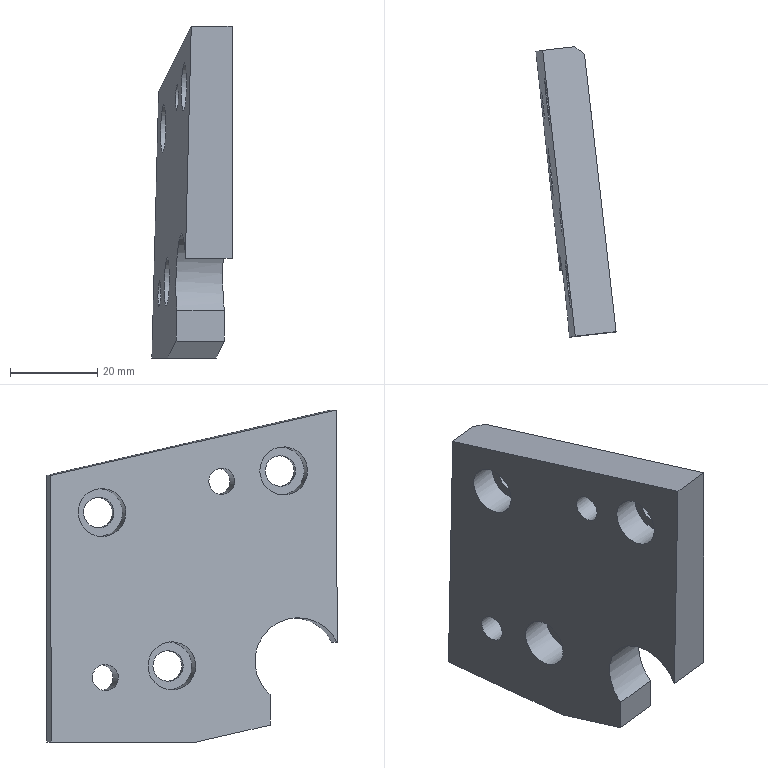Part | NX | features XQ 2 | 1 solid | 21 faces | box 18.384 x 66.57 x 76.127 mm | volume 38199 mm3 | plane 12 | cylinder 9 | commonest cylinder face diameters 7 x3 11 x3 6.001 x2 20 x1
STEP:
#1=CARTESIAN_POINT('',(2648.067,365.159,-95.222));
#2=VERTEX_POINT('',#1);
#3=CARTESIAN_POINT('',(2647.727,368.14,-95.222));
#4=DIRECTION('',(-0.9936,-0.1132,-0.000000001));
#5=DIRECTION('',(0.1132,-0.9936,0.));
#6=AXIS2_PLACEMENT_3D('',#3,#4,#5);
#7=CIRCLE('',#6,3.001);
#8=EDGE_CURVE('',#2,#2,#7,.T.);
#9=ORIENTED_EDGE('',*,*,#8,.F.);
#10=EDGE_LOOP('',(#9));
#11=FACE_BOUND('',#10,.T.);
#12=CARTESIAN_POINT('',(2637.119,367.602,-92.296));
#13=VERTEX_POINT('',#12);
#14=CARTESIAN_POINT('',(2637.116,366.931,-95.222));
#15=DIRECTION('',(-0.9939,-0.1074,0.02552));
#16=DIRECTION('',(0.0008715,0.2236,0.9747));
#17=AXIS2_PLACEMENT_3D('',#14,#15,#16);
#18=ELLIPSE('',#17,3.002,3.001);
#19=EDGE_CURVE('',#13,#13,#18,.T.);
#20=ORIENTED_EDGE('',*,*,#19,.T.);
#21=EDGE_LOOP('',(#20));
#22=FACE_BOUND('',#21,.T.);
#23=CARTESIAN_POINT('',(2635.804,366.781,-95.222));
#24=DIRECTION('',(0.9936,0.1132,0.));
#25=DIRECTION('',(-0.01281,0.1125,-0.9936));
#26=AXIS2_PLACEMENT_3D('',#23,#24,#25);
#27=CYLINDRICAL_SURFACE('',#26,3.001);
#28=ADVANCED_FACE('',(#11,#22),#27,.F.);
#29=CARTESIAN_POINT('',(2646.439,352.939,-96.027));
#30=VERTEX_POINT('',#29);
#31=CARTESIAN_POINT('',(2646.484,352.545,-92.549));
#32=DIRECTION('',(-0.9936,-0.1132,0.));
#33=DIRECTION('',(-0.01281,0.1125,-0.9936));
#34=AXIS2_PLACEMENT_3D('',#31,#32,#33);
#35=CIRCLE('',#34,3.5);
#36=EDGE_CURVE('',#30,#30,#35,.T.);
#37=ORIENTED_EDGE('',*,*,#36,.F.);
#38=EDGE_LOOP('',(#37));
#39=FACE_BOUND('',#38,.T.);
#40=CARTESIAN_POINT('',(2646.555,351.926,-87.085));
#41=VERTEX_POINT('',#40);
#42=CARTESIAN_POINT('',(2646.484,352.545,-92.549));
#43=DIRECTION('',(-0.9936,-0.1132,0.));
#44=DIRECTION('',(0.01281,-0.1125,0.9936));
#45=AXIS2_PLACEMENT_3D('',#42,#43,#44);
#46=CIRCLE('',#45,5.5);
#47=EDGE_CURVE('',#41,#41,#46,.T.);
#48=ORIENTED_EDGE('',*,*,#47,.T.);
#49=EDGE_LOOP('',(#48));
#50=FACE_BOUND('',#49,.T.);
#51=CARTESIAN_POINT('',(2646.484,352.545,-92.549));
#52=DIRECTION('',(0.9936,0.1132,0.));
#53=DIRECTION('',(0.01281,-0.1125,0.9936));
#54=AXIS2_PLACEMENT_3D('',#51,#52,#53);
#55=PLANE('',#54);
#56=ADVANCED_FACE('',(#39,#50),#55,.F.);
#57=CARTESIAN_POINT('',(2644.627,368.844,-60.872));
#58=VERTEX_POINT('',#57);
#59=CARTESIAN_POINT('',(2644.672,368.45,-57.395));
#60=DIRECTION('',(-0.9936,-0.1132,0.));
#61=DIRECTION('',(-0.01281,0.1125,-0.9936));
#62=AXIS2_PLACEMENT_3D('',#59,#60,#61);
#63=CIRCLE('',#62,3.5);
#64=EDGE_CURVE('',#58,#58,#63,.T.);
#65=ORIENTED_EDGE('',*,*,#64,.F.);
#66=EDGE_LOOP('',(#65));
#67=FACE_BOUND('',#66,.T.);
#68=CARTESIAN_POINT('',(2644.743,367.831,-51.93));
#69=VERTEX_POINT('',#68);
#70=CARTESIAN_POINT('',(2644.672,368.45,-57.395));
#71=DIRECTION('',(-0.9936,-0.1132,0.));
#72=DIRECTION('',(0.01281,-0.1125,0.9936));
#73=AXIS2_PLACEMENT_3D('',#70,#71,#72);
#74=CIRCLE('',#73,5.5);
#75=EDGE_CURVE('',#69,#69,#74,.T.);
#76=ORIENTED_EDGE('',*,*,#75,.T.);
#77=EDGE_LOOP('',(#76));
#78=FACE_BOUND('',#77,.T.);
#79=CARTESIAN_POINT('',(2644.672,368.45,-57.395));
#80=DIRECTION('',(0.9936,0.1132,0.));
#81=DIRECTION('',(0.01281,-0.1125,0.9936));
#82=AXIS2_PLACEMENT_3D('',#79,#80,#81);
#83=PLANE('',#82);
#84=ADVANCED_FACE('',(#67,#78),#83,.F.);
#85=CARTESIAN_POINT('',(2649.373,327.188,-51.321));
#86=VERTEX_POINT('',#85);
#87=CARTESIAN_POINT('',(2649.418,326.794,-47.843));
#88=DIRECTION('',(-0.9936,-0.1132,0.));
#89=DIRECTION('',(-0.01281,0.1125,-0.9936));
#90=AXIS2_PLACEMENT_3D('',#87,#88,#89);
#91=CIRCLE('',#90,3.5);
#92=EDGE_CURVE('',#86,#86,#91,.T.);
#93=ORIENTED_EDGE('',*,*,#92,.F.);
#94=EDGE_LOOP('',(#93));
#95=FACE_BOUND('',#94,.T.);
#96=CARTESIAN_POINT('',(2649.489,326.175,-42.378));
#97=VERTEX_POINT('',#96);
#98=CARTESIAN_POINT('',(2649.418,326.794,-47.843));
#99=DIRECTION('',(-0.9936,-0.1132,0.));
#100=DIRECTION('',(0.01281,-0.1125,0.9936));
#101=AXIS2_PLACEMENT_3D('',#98,#99,#100);
#102=CIRCLE('',#101,5.5);
#103=EDGE_CURVE('',#97,#97,#102,.T.);
#104=ORIENTED_EDGE('',*,*,#103,.T.);
#105=EDGE_LOOP('',(#104));
#106=FACE_BOUND('',#105,.T.);
#107=CARTESIAN_POINT('',(2647.873,340.356,-50.953));
#108=DIRECTION('',(0.9936,0.1132,0.));
#109=DIRECTION('',(0.01281,-0.1125,0.9936));
#110=AXIS2_PLACEMENT_3D('',#107,#108,#109);
#111=PLANE('',#110);
#112=ADVANCED_FACE('',(#95,#106),#111,.F.);
#113=CARTESIAN_POINT('',(2649.861,349.407,-92.549));
#114=VERTEX_POINT('',#113);
#115=CARTESIAN_POINT('',(2649.465,352.885,-92.549));
#116=DIRECTION('',(-0.9936,-0.1132,-0.000000001));
#117=DIRECTION('',(0.1132,-0.9936,0.));
#118=AXIS2_PLACEMENT_3D('',#115,#116,#117);
#119=CIRCLE('',#118,3.5);
#120=EDGE_CURVE('',#114,#114,#119,.T.);
#121=ORIENTED_EDGE('',*,*,#120,.F.);
#122=EDGE_LOOP('',(#121));
#123=FACE_BOUND('',#122,.T.);
#124=ORIENTED_EDGE('',*,*,#36,.T.);
#125=EDGE_LOOP('',(#124));
#126=FACE_BOUND('',#125,.T.);
#127=CARTESIAN_POINT('',(2637.542,351.526,-92.549));
#128=DIRECTION('',(0.9936,0.1132,0.));
#129=DIRECTION('',(-0.01281,0.1125,-0.9936));
#130=AXIS2_PLACEMENT_3D('',#127,#128,#129);
#131=CYLINDRICAL_SURFACE('',#130,3.5);
#132=ADVANCED_FACE('',(#123,#126),#131,.F.);
#133=CARTESIAN_POINT('',(2648.049,365.312,-57.395));
#134=VERTEX_POINT('',#133);
#135=CARTESIAN_POINT('',(2647.653,368.79,-57.395));
#136=DIRECTION('',(-0.9936,-0.1132,-0.000000001));
#137=DIRECTION('',(0.1132,-0.9936,0.));
#138=AXIS2_PLACEMENT_3D('',#135,#136,#137);
#139=CIRCLE('',#138,3.5);
#140=EDGE_CURVE('',#134,#134,#139,.T.);
#141=ORIENTED_EDGE('',*,*,#140,.F.);
#142=EDGE_LOOP('',(#141));
#143=FACE_BOUND('',#142,.T.);
#144=ORIENTED_EDGE('',*,*,#64,.T.);
#145=EDGE_LOOP('',(#144));
#146=FACE_BOUND('',#145,.T.);
#147=CARTESIAN_POINT('',(2635.73,367.431,-57.395));
#148=DIRECTION('',(0.9936,0.1132,0.));
#149=DIRECTION('',(-0.01281,0.1125,-0.9936));
#150=AXIS2_PLACEMENT_3D('',#147,#148,#149);
#151=CYLINDRICAL_SURFACE('',#150,3.5);
#152=ADVANCED_FACE('',(#143,#146),#151,.F.);
#153=CARTESIAN_POINT('',(2644.323,380.35,-48.909));
#154=VERTEX_POINT('',#153);
#155=CARTESIAN_POINT('',(2636.947,379.51,-48.909));
#156=VERTEX_POINT('',#155);
#157=CARTESIAN_POINT('',(2651.278,381.143,-48.909));
#158=DIRECTION('',(-0.9936,-0.1132,-0.000000001));
#159=VECTOR('',#158,1000.);
#160=LINE('',#157,#159);
#161=EDGE_CURVE('',#154,#156,#160,.T.);
#162=ORIENTED_EDGE('',*,*,#161,.F.);
#163=CARTESIAN_POINT('',(2644.323,380.35,-110.));
#164=VERTEX_POINT('',#163);
#165=CARTESIAN_POINT('',(2644.323,380.35,-0.00000008));
#166=DIRECTION('',(0.000000001,0.,-1.));
#167=VECTOR('',#166,1000.);
#168=LINE('',#165,#167);
#169=EDGE_CURVE('',#154,#164,#168,.T.);
#170=ORIENTED_EDGE('',*,*,#169,.T.);
#171=CARTESIAN_POINT('',(2635.397,379.333,-110.));
#172=VERTEX_POINT('',#171);
#173=CARTESIAN_POINT('',(2651.278,381.143,-110.));
#174=DIRECTION('',(0.9936,0.1132,0.));
#175=VECTOR('',#174,1000.);
#176=LINE('',#173,#175);
#177=EDGE_CURVE('',#172,#164,#176,.T.);
#178=ORIENTED_EDGE('',*,*,#177,.F.);
#179=CARTESIAN_POINT('',(2638.196,379.652,0.3362));
#180=DIRECTION('',(0.02536,0.002889,0.9997));
#181=VECTOR('',#180,1000.);
#182=LINE('',#179,#181);
#183=EDGE_CURVE('',#172,#156,#182,.T.);
#184=ORIENTED_EDGE('',*,*,#183,.T.);
#185=EDGE_LOOP('',(#162,#170,#178,#184));
#186=FACE_BOUND('',#185,.T.);
#187=CARTESIAN_POINT('',(2651.278,381.143,-0.000000075));
#188=DIRECTION('',(0.1132,-0.9936,0.));
#189=DIRECTION('',(0.9936,0.1132,0.));
#190=AXIS2_PLACEMENT_3D('',#187,#188,#189);
#191=PLANE('',#190);
#192=ADVANCED_FACE('',(#186),#191,.F.);
#193=ORIENTED_EDGE('',*,*,#177,.T.);
#194=CARTESIAN_POINT('',(2646.536,378.59,-110.));
#195=VERTEX_POINT('',#194);
#196=CARTESIAN_POINT('',(2389.056,583.399,-110.));
#197=DIRECTION('',(0.7826,-0.6225,0.));
#198=VECTOR('',#197,1000.);
#199=LINE('',#196,#198);
#200=EDGE_CURVE('',#164,#195,#199,.T.);
#201=ORIENTED_EDGE('',*,*,#200,.T.);
#202=CARTESIAN_POINT('',(2650.099,347.318,-110.));
#203=VERTEX_POINT('',#202);
#204=CARTESIAN_POINT('',(2511.71,1561.949,-110.));
#205=DIRECTION('',(0.1132,-0.9936,0.));
#206=VECTOR('',#205,1000.);
#207=LINE('',#204,#206);
#208=EDGE_CURVE('',#195,#203,#207,.T.);
#209=ORIENTED_EDGE('',*,*,#208,.T.);
#210=CARTESIAN_POINT('',(2638.993,346.053,-110.));
#211=VERTEX_POINT('',#210);
#212=CARTESIAN_POINT('',(1895.227,261.312,-110.));
#213=DIRECTION('',(0.9936,0.1132,0.));
#214=VECTOR('',#213,1000.);
#215=LINE('',#212,#214);
#216=EDGE_CURVE('',#211,#203,#215,.T.);
#217=ORIENTED_EDGE('',*,*,#216,.F.);
#218=CARTESIAN_POINT('',(2507.675,1561.427,-110.));
#219=DIRECTION('',(0.1074,-0.9942,0.));
#220=VECTOR('',#219,1000.);
#221=LINE('',#218,#220);
#222=EDGE_CURVE('',#172,#211,#221,.T.);
#223=ORIENTED_EDGE('',*,*,#222,.F.);
#224=EDGE_LOOP('',(#193,#201,#209,#217,#223));
#225=FACE_BOUND('',#224,.T.);
#226=CARTESIAN_POINT('',(1925.,0.,-110.));
#227=DIRECTION('',(0.,0.,-1.));
#228=DIRECTION('',(1.,0.,0.));
#229=AXIS2_PLACEMENT_3D('',#226,#227,#228);
#230=PLANE('',#229);
#231=ADVANCED_FACE('',(#225),#230,.T.);
#232=CARTESIAN_POINT('',(2640.92,329.136,-106.121));
#233=VERTEX_POINT('',#232);
#234=CARTESIAN_POINT('',(2652.027,330.401,-106.121));
#235=VERTEX_POINT('',#234);
#236=CARTESIAN_POINT('',(2647.059,329.835,-106.121));
#237=DIRECTION('',(0.9936,0.1132,0.000000001));
#238=VECTOR('',#237,1000.);
#239=LINE('',#236,#238);
#240=EDGE_CURVE('',#233,#235,#239,.T.);
#241=ORIENTED_EDGE('',*,*,#240,.F.);
#242=CARTESIAN_POINT('',(2492.804,1629.133,-404.205));
#243=DIRECTION('',(0.1104,-0.9687,0.2221));
#244=VECTOR('',#243,1000.);
#245=LINE('',#242,#244);
#246=EDGE_CURVE('',#211,#233,#245,.T.);
#247=ORIENTED_EDGE('',*,*,#246,.F.);
#248=ORIENTED_EDGE('',*,*,#216,.T.);
#249=CARTESIAN_POINT('',(2503.911,1630.398,-404.205));
#250=DIRECTION('',(0.1104,-0.9687,0.2221));
#251=VECTOR('',#250,1000.);
#252=LINE('',#249,#251);
#253=EDGE_CURVE('',#203,#235,#252,.T.);
#254=ORIENTED_EDGE('',*,*,#253,.T.);
#255=EDGE_LOOP('',(#241,#247,#248,#254));
#256=FACE_BOUND('',#255,.T.);
#257=CARTESIAN_POINT('',(2652.739,302.066,-99.689));
#258=DIRECTION('',(0.02515,-0.2207,-0.975));
#259=DIRECTION('',(0.,0.9753,-0.2208));
#260=AXIS2_PLACEMENT_3D('',#257,#258,#259);
#261=PLANE('',#260);
#262=ADVANCED_FACE('',(#256),#261,.T.);
#263=ORIENTED_EDGE('',*,*,#240,.T.);
#264=CARTESIAN_POINT('',(2652.027,330.401,-99.099));
#265=VERTEX_POINT('',#264);
#266=CARTESIAN_POINT('',(2652.027,330.401,-706.6));
#267=DIRECTION('',(-0.000000001,0.,1.));
#268=VECTOR('',#267,1000.);
#269=LINE('',#266,#268);
#270=EDGE_CURVE('',#235,#265,#269,.T.);
#271=ORIENTED_EDGE('',*,*,#270,.T.);
#272=CARTESIAN_POINT('',(2641.098,329.156,-99.099));
#273=VERTEX_POINT('',#272);
#274=CARTESIAN_POINT('',(2642.091,329.269,-99.099));
#275=DIRECTION('',(0.9936,0.1132,0.000000001));
#276=VECTOR('',#275,1000.);
#277=LINE('',#274,#276);
#278=EDGE_CURVE('',#273,#265,#277,.T.);
#279=ORIENTED_EDGE('',*,*,#278,.F.);
#280=CARTESIAN_POINT('',(2625.695,327.401,-706.297));
#281=DIRECTION('',(-0.02536,-0.002889,-0.9997));
#282=VECTOR('',#281,1000.);
#283=LINE('',#280,#282);
#284=EDGE_CURVE('',#273,#233,#283,.T.);
#285=ORIENTED_EDGE('',*,*,#284,.T.);
#286=EDGE_LOOP('',(#263,#271,#279,#285));
#287=FACE_BOUND('',#286,.T.);
#288=CARTESIAN_POINT('',(2647.059,329.835,-79.455));
#289=DIRECTION('',(-0.1132,0.9936,0.));
#290=DIRECTION('',(-0.9936,-0.1132,0.));
#291=AXIS2_PLACEMENT_3D('',#288,#289,#290);
#292=PLANE('',#291);
#293=ADVANCED_FACE('',(#287),#292,.F.);
#294=CARTESIAN_POINT('',(2653.781,315.001,-87.141));
#295=VERTEX_POINT('',#294);
#296=CARTESIAN_POINT('',(2643.067,313.78,-87.141));
#297=VERTEX_POINT('',#296);
#298=CARTESIAN_POINT('',(3066.114,361.98,-87.141));
#299=DIRECTION('',(-0.9936,-0.1132,-0.000000001));
#300=VECTOR('',#299,1000.);
#301=LINE('',#298,#300);
#302=EDGE_CURVE('',#295,#297,#301,.T.);
#303=ORIENTED_EDGE('',*,*,#302,.T.);
#304=CARTESIAN_POINT('',(2641.989,322.716,-91.5));
#305=DIRECTION('',(-0.9939,-0.1074,0.02552));
#306=DIRECTION('',(-0.0008715,-0.2236,-0.9747));
#307=AXIS2_PLACEMENT_3D('',#304,#305,#306);
#308=ELLIPSE('',#307,10.003,10.);
#309=EDGE_CURVE('',#297,#273,#308,.T.);
#310=ORIENTED_EDGE('',*,*,#309,.T.);
#311=ORIENTED_EDGE('',*,*,#278,.T.);
#312=CARTESIAN_POINT('',(2652.762,323.943,-91.5));
#313=DIRECTION('',(-0.9936,-0.1132,-0.000000001));
#314=DIRECTION('',(0.000000001,0.,-1.));
#315=AXIS2_PLACEMENT_3D('',#312,#313,#314);
#316=CIRCLE('',#315,10.);
#317=EDGE_CURVE('',#295,#265,#316,.T.);
#318=ORIENTED_EDGE('',*,*,#317,.F.);
#319=EDGE_LOOP('',(#303,#310,#311,#318));
#320=FACE_BOUND('',#319,.T.);
#321=CARTESIAN_POINT('',(3065.095,370.923,-91.5));
#322=DIRECTION('',(-0.9936,-0.1132,-0.000000001));
#323=DIRECTION('',(0.000000001,0.,-1.));
#324=AXIS2_PLACEMENT_3D('',#321,#322,#323);
#325=CYLINDRICAL_SURFACE('',#324,10.);
#326=ADVANCED_FACE('',(#320),#325,.F.);
#327=CARTESIAN_POINT('',(2653.781,315.001,-33.873));
#328=VERTEX_POINT('',#327);
#329=CARTESIAN_POINT('',(2653.781,315.001,-706.6));
#330=DIRECTION('',(-0.000000001,0.,1.));
#331=VECTOR('',#330,1000.);
#332=LINE('',#329,#331);
#333=EDGE_CURVE('',#295,#328,#332,.T.);
#334=ORIENTED_EDGE('',*,*,#333,.T.);
#335=CARTESIAN_POINT('',(2644.418,313.934,-33.873));
#336=VERTEX_POINT('',#335);
#337=CARTESIAN_POINT('',(2658.749,315.567,-33.873));
#338=DIRECTION('',(0.9936,0.1132,0.000000001));
#339=VECTOR('',#338,1000.);
#340=LINE('',#337,#339);
#341=EDGE_CURVE('',#336,#328,#340,.T.);
#342=ORIENTED_EDGE('',*,*,#341,.F.);
#343=CARTESIAN_POINT('',(2627.36,311.991,-706.295));
#344=DIRECTION('',(-0.02536,-0.002889,-0.9997));
#345=VECTOR('',#344,1000.);
#346=LINE('',#343,#345);
#347=EDGE_CURVE('',#336,#297,#346,.T.);
#348=ORIENTED_EDGE('',*,*,#347,.T.);
#349=ORIENTED_EDGE('',*,*,#302,.F.);
#350=EDGE_LOOP('',(#334,#342,#348,#349));
#351=FACE_BOUND('',#350,.T.);
#352=CARTESIAN_POINT('',(2648.813,314.435,-79.455));
#353=DIRECTION('',(-0.1132,0.9936,0.));
#354=DIRECTION('',(-0.9936,-0.1132,0.));
#355=AXIS2_PLACEMENT_3D('',#352,#353,#354);
#356=PLANE('',#355);
#357=ADVANCED_FACE('',(#351),#356,.F.);
#358=CARTESIAN_POINT('',(2646.536,378.59,-48.454));
#359=VERTEX_POINT('',#358);
#360=CARTESIAN_POINT('',(2502.226,1645.185,-338.879));
#361=DIRECTION('',(0.1104,-0.9687,0.2221));
#362=VECTOR('',#361,1000.);
#363=LINE('',#360,#362);
#364=EDGE_CURVE('',#359,#328,#363,.T.);
#365=ORIENTED_EDGE('',*,*,#364,.F.);
#366=CARTESIAN_POINT('',(2565.66,442.922,-65.101));
#367=DIRECTION('',(-0.7726,0.6146,-0.159));
#368=VECTOR('',#367,1000.);
#369=LINE('',#366,#368);
#370=EDGE_CURVE('',#359,#154,#369,.T.);
#371=ORIENTED_EDGE('',*,*,#370,.T.);
#372=ORIENTED_EDGE('',*,*,#161,.T.);
#373=CARTESIAN_POINT('',(2492.863,1644.118,-338.879));
#374=DIRECTION('',(0.1104,-0.9687,0.2221));
#375=VECTOR('',#374,1000.);
#376=LINE('',#373,#375);
#377=EDGE_CURVE('',#156,#336,#376,.T.);
#378=ORIENTED_EDGE('',*,*,#377,.T.);
#379=ORIENTED_EDGE('',*,*,#341,.T.);
#380=EDGE_LOOP('',(#365,#371,#372,#378,#379));
#381=FACE_BOUND('',#380,.T.);
#382=CARTESIAN_POINT('',(2659.211,311.513,-32.943));
#383=DIRECTION('',(-0.02515,0.2207,0.975));
#384=DIRECTION('',(0.,-0.9753,0.2208));
#385=AXIS2_PLACEMENT_3D('',#382,#383,#384);
#386=PLANE('',#385);
#387=ADVANCED_FACE('',(#381),#386,.T.);
#388=CARTESIAN_POINT('',(2651.123,338.332,-50.222));
#389=VERTEX_POINT('',#388);
#390=CARTESIAN_POINT('',(2650.783,341.313,-50.222));
#391=DIRECTION('',(-0.9936,-0.1132,-0.000000001));
#392=DIRECTION('',(0.1132,-0.9936,0.));
#393=AXIS2_PLACEMENT_3D('',#390,#391,#392);
#394=CIRCLE('',#393,3.001);
#395=EDGE_CURVE('',#389,#389,#394,.T.);
#396=ORIENTED_EDGE('',*,*,#395,.F.);
#397=EDGE_LOOP('',(#396));
#398=FACE_BOUND('',#397,.T.);
#399=CARTESIAN_POINT('',(2641.161,340.888,-47.296));
#400=VERTEX_POINT('',#399);
#401=CARTESIAN_POINT('',(2641.158,340.217,-50.222));
#402=DIRECTION('',(-0.9939,-0.1074,0.02552));
#403=DIRECTION('',(0.0008715,0.2236,0.9747));
#404=AXIS2_PLACEMENT_3D('',#401,#402,#403);
#405=ELLIPSE('',#404,3.002,3.001);
#406=EDGE_CURVE('',#400,#400,#405,.T.);
#407=ORIENTED_EDGE('',*,*,#406,.T.);
#408=EDGE_LOOP('',(#407));
#409=FACE_BOUND('',#408,.T.);
#410=CARTESIAN_POINT('',(2638.86,339.955,-50.222));
#411=DIRECTION('',(0.9936,0.1132,0.));
#412=DIRECTION('',(-0.01281,0.1125,-0.9936));
#413=AXIS2_PLACEMENT_3D('',#410,#411,#412);
#414=CYLINDRICAL_SURFACE('',#413,3.001);
#415=ADVANCED_FACE('',(#398,#409),#414,.F.);
#416=ORIENTED_EDGE('',*,*,#47,.F.);
#417=EDGE_LOOP('',(#416));
#418=FACE_BOUND('',#417,.T.);
#419=CARTESIAN_POINT('',(2638.838,352.903,-87.187));
#420=VERTEX_POINT('',#419);
#421=CARTESIAN_POINT('',(2638.834,351.673,-92.549));
#422=DIRECTION('',(-0.9939,-0.1074,0.02552));
#423=DIRECTION('',(0.0008715,0.2236,0.9747));
#424=AXIS2_PLACEMENT_3D('',#421,#422,#423);
#425=ELLIPSE('',#424,5.502,5.5);
#426=EDGE_CURVE('',#420,#420,#425,.T.);
#427=ORIENTED_EDGE('',*,*,#426,.T.);
#428=EDGE_LOOP('',(#427));
#429=FACE_BOUND('',#428,.T.);
#430=CARTESIAN_POINT('',(2639.529,351.753,-92.549));
#431=DIRECTION('',(0.9936,0.1132,0.));
#432=DIRECTION('',(-0.01281,0.1125,-0.9936));
#433=AXIS2_PLACEMENT_3D('',#430,#431,#432);
#434=CYLINDRICAL_SURFACE('',#433,5.5);
#435=ADVANCED_FACE('',(#418,#429),#434,.F.);
#436=ORIENTED_EDGE('',*,*,#75,.F.);
#437=EDGE_LOOP('',(#436));
#438=FACE_BOUND('',#437,.T.);
#439=CARTESIAN_POINT('',(2638.01,368.921,-52.032));
#440=VERTEX_POINT('',#439);
#441=CARTESIAN_POINT('',(2638.006,367.691,-57.395));
#442=DIRECTION('',(-0.9939,-0.1074,0.02552));
#443=DIRECTION('',(0.0008715,0.2236,0.9747));
#444=AXIS2_PLACEMENT_3D('',#441,#442,#443);
#445=ELLIPSE('',#444,5.502,5.5);
#446=EDGE_CURVE('',#440,#440,#445,.T.);
#447=ORIENTED_EDGE('',*,*,#446,.T.);
#448=EDGE_LOOP('',(#447));
#449=FACE_BOUND('',#448,.T.);
#450=CARTESIAN_POINT('',(2637.717,367.658,-57.395));
#451=DIRECTION('',(0.9936,0.1132,0.));
#452=DIRECTION('',(-0.01281,0.1125,-0.9936));
#453=AXIS2_PLACEMENT_3D('',#450,#451,#452);
#454=CYLINDRICAL_SURFACE('',#453,5.5);
#455=ADVANCED_FACE('',(#438,#449),#454,.F.);
#456=ORIENTED_EDGE('',*,*,#103,.F.);
#457=EDGE_LOOP('',(#456));
#458=FACE_BOUND('',#457,.T.);
#459=CARTESIAN_POINT('',(2642.757,327.264,-42.481));
#460=VERTEX_POINT('',#459);
#461=CARTESIAN_POINT('',(2642.752,326.034,-47.843));
#462=DIRECTION('',(-0.9939,-0.1074,0.02552));
#463=DIRECTION('',(0.0008715,0.2236,0.9747));
#464=AXIS2_PLACEMENT_3D('',#461,#462,#463);
#465=ELLIPSE('',#464,5.502,5.5);
#466=EDGE_CURVE('',#460,#460,#465,.T.);
#467=ORIENTED_EDGE('',*,*,#466,.T.);
#468=EDGE_LOOP('',(#467));
#469=FACE_BOUND('',#468,.T.);
#470=CARTESIAN_POINT('',(2642.463,326.001,-47.843));
#471=DIRECTION('',(0.9936,0.1132,0.));
#472=DIRECTION('',(-0.01281,0.1125,-0.9936));
#473=AXIS2_PLACEMENT_3D('',#470,#471,#472);
#474=CYLINDRICAL_SURFACE('',#473,5.5);
#475=ADVANCED_FACE('',(#458,#469),#474,.F.);
#476=ORIENTED_EDGE('',*,*,#19,.F.);
#477=EDGE_LOOP('',(#476));
#478=FACE_BOUND('',#477,.T.);
#479=ORIENTED_EDGE('',*,*,#466,.F.);
#480=EDGE_LOOP('',(#479));
#481=FACE_BOUND('',#480,.T.);
#482=ORIENTED_EDGE('',*,*,#446,.F.);
#483=EDGE_LOOP('',(#482));
#484=FACE_BOUND('',#483,.T.);
#485=ORIENTED_EDGE('',*,*,#426,.F.);
#486=EDGE_LOOP('',(#485));
#487=FACE_BOUND('',#486,.T.);
#488=ORIENTED_EDGE('',*,*,#406,.F.);
#489=EDGE_LOOP('',(#488));
#490=FACE_BOUND('',#489,.T.);
#491=ORIENTED_EDGE('',*,*,#377,.F.);
#492=ORIENTED_EDGE('',*,*,#183,.F.);
#493=ORIENTED_EDGE('',*,*,#222,.T.);
#494=ORIENTED_EDGE('',*,*,#246,.T.);
#495=ORIENTED_EDGE('',*,*,#284,.F.);
#496=ORIENTED_EDGE('',*,*,#309,.F.);
#497=ORIENTED_EDGE('',*,*,#347,.F.);
#498=EDGE_LOOP('',(#491,#492,#493,#494,#495,#496,#497));
#499=FACE_BOUND('',#498,.T.);
#500=CARTESIAN_POINT('',(2492.534,1559.791,-706.481));
#501=DIRECTION('',(0.9939,0.1074,-0.02552));
#502=DIRECTION('',(-0.02537,-0.002816,-0.9997));
#503=AXIS2_PLACEMENT_3D('',#500,#501,#502);
#504=PLANE('',#503);
#505=ADVANCED_FACE('',(#478,#481,#484,#487,#490,#499),#504,.F.);
#506=CARTESIAN_POINT('',(2652.795,323.656,-47.843));
#507=VERTEX_POINT('',#506);
#508=CARTESIAN_POINT('',(2652.399,327.133,-47.843));
#509=DIRECTION('',(-0.9936,-0.1132,-0.000000001));
#510=DIRECTION('',(0.1132,-0.9936,0.));
#511=AXIS2_PLACEMENT_3D('',#508,#509,#510);
#512=CIRCLE('',#511,3.5);
#513=EDGE_CURVE('',#507,#507,#512,.T.);
#514=ORIENTED_EDGE('',*,*,#513,.F.);
#515=EDGE_LOOP('',(#514));
#516=FACE_BOUND('',#515,.T.);
#517=ORIENTED_EDGE('',*,*,#92,.T.);
#518=EDGE_LOOP('',(#517));
#519=FACE_BOUND('',#518,.T.);
#520=CARTESIAN_POINT('',(2640.476,325.775,-47.843));
#521=DIRECTION('',(0.9936,0.1132,0.));
#522=DIRECTION('',(-0.01281,0.1125,-0.9936));
#523=AXIS2_PLACEMENT_3D('',#520,#521,#522);
#524=CYLINDRICAL_SURFACE('',#523,3.5);
#525=ADVANCED_FACE('',(#516,#519),#524,.F.);
#526=ORIENTED_EDGE('',*,*,#8,.T.);
#527=EDGE_LOOP('',(#526));
#528=FACE_BOUND('',#527,.T.);
#529=ORIENTED_EDGE('',*,*,#513,.T.);
#530=EDGE_LOOP('',(#529));
#531=FACE_BOUND('',#530,.T.);
#532=ORIENTED_EDGE('',*,*,#208,.F.);
#533=CARTESIAN_POINT('',(2646.536,378.59,-706.6));
#534=DIRECTION('',(-0.000000001,0.,1.));
#535=VECTOR('',#534,1000.);
#536=LINE('',#533,#535);
#537=EDGE_CURVE('',#195,#359,#536,.T.);
#538=ORIENTED_EDGE('',*,*,#537,.T.);
#539=ORIENTED_EDGE('',*,*,#364,.T.);
#540=ORIENTED_EDGE('',*,*,#333,.F.);
#541=ORIENTED_EDGE('',*,*,#317,.T.);
#542=ORIENTED_EDGE('',*,*,#270,.F.);
#543=ORIENTED_EDGE('',*,*,#253,.F.);
#544=EDGE_LOOP('',(#532,#538,#539,#540,#541,#542,#543));
#545=FACE_BOUND('',#544,.T.);
#546=ORIENTED_EDGE('',*,*,#140,.T.);
#547=EDGE_LOOP('',(#546));
#548=FACE_BOUND('',#547,.T.);
#549=ORIENTED_EDGE('',*,*,#120,.T.);
#550=EDGE_LOOP('',(#549));
#551=FACE_BOUND('',#550,.T.);
#552=ORIENTED_EDGE('',*,*,#395,.T.);
#553=EDGE_LOOP('',(#552));
#554=FACE_BOUND('',#553,.T.);
#555=CARTESIAN_POINT('',(2511.71,1561.949,-706.6));
#556=DIRECTION('',(0.9936,0.1132,0.000000001));
#557=DIRECTION('',(0.000000001,-0.000000001,-1.));
#558=AXIS2_PLACEMENT_3D('',#555,#556,#557);
#559=PLANE('',#558);
#560=ADVANCED_FACE('',(#528,#531,#545,#548,#551,#554),#559,.T.);
#561=ORIENTED_EDGE('',*,*,#200,.F.);
#562=ORIENTED_EDGE('',*,*,#169,.F.);
#563=ORIENTED_EDGE('',*,*,#370,.F.);
#564=ORIENTED_EDGE('',*,*,#537,.F.);
#565=EDGE_LOOP('',(#561,#562,#563,#564));
#566=FACE_BOUND('',#565,.T.);
#567=CARTESIAN_POINT('',(2646.536,378.59,-706.6));
#568=DIRECTION('',(0.6225,0.7826,0.));
#569=DIRECTION('',(-0.000000001,0.,1.));
#570=AXIS2_PLACEMENT_3D('',#567,#568,#569);
#571=PLANE('',#570);
#572=ADVANCED_FACE('',(#566),#571,.T.);
#573=CLOSED_SHELL('',(#28,#56,#84,#112,#132,#152,#192,#231,#262,#293,#326,#357,#387,#415,#435,#455,#475,#505,#525,#560,#572));
#574=MANIFOLD_SOLID_BREP('',#573);
#575=(LENGTH_UNIT()NAMED_UNIT(*)SI_UNIT(.MILLI.,.METRE.));
#576=UNCERTAINTY_MEASURE_WITH_UNIT(LENGTH_MEASURE(0.00001),#575,'','');
#577=(NAMED_UNIT(*)PLANE_ANGLE_UNIT()SI_UNIT($,.RADIAN.));
#578=(NAMED_UNIT(*)SI_UNIT($,.STERADIAN.)SOLID_ANGLE_UNIT());
#579=(GEOMETRIC_REPRESENTATION_CONTEXT(3)GLOBAL_UNCERTAINTY_ASSIGNED_CONTEXT((#576))GLOBAL_UNIT_ASSIGNED_CONTEXT((#575,#577,#578))REPRESENTATION_CONTEXT('',''));
#580=ADVANCED_BREP_SHAPE_REPRESENTATION('',(#574),#579);